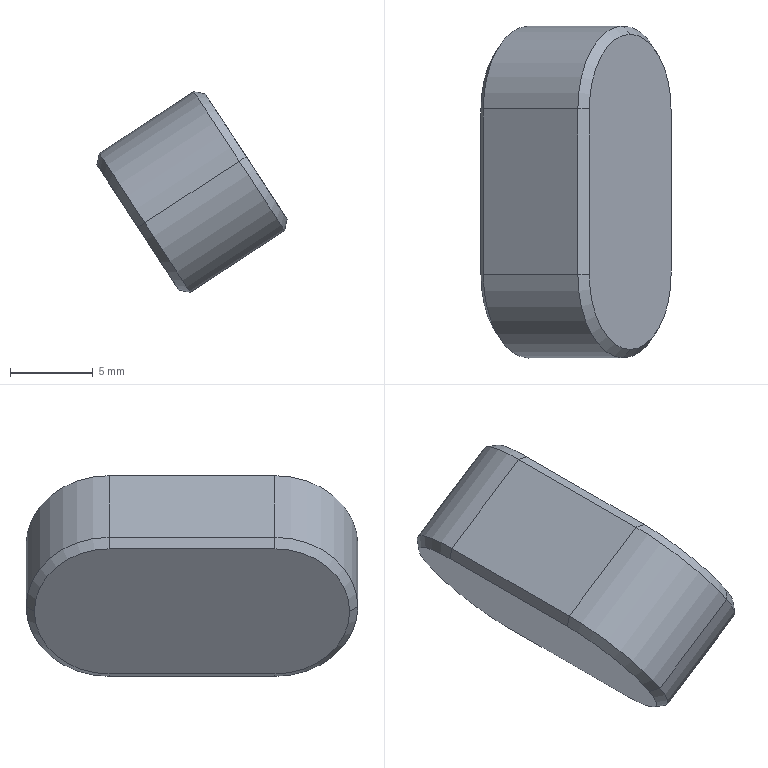Part | NX | features BREP 1 | 1 solid | 20 faces | box 11.452 x 20 x 12.091 mm | volume 1380 mm3 | plane 8 | cone 8 | cylinder 4 | commonest cylinder face diameters 10 x4
STEP:
#1=CARTESIAN_POINT('',(143.048,321.,299.856));
#2=VERTEX_POINT('',#1);
#3=CARTESIAN_POINT('',(140.587,325.5,303.624));
#4=VERTEX_POINT('',#3);
#5=CARTESIAN_POINT('',(140.587,321.,303.624));
#6=DIRECTION('',(0.8372,0.,0.5469));
#7=DIRECTION('',(0.5469,0.,-0.8372));
#8=AXIS2_PLACEMENT_3D('',#5,#6,#7);
#9=CIRCLE('',#8,4.5);
#10=EDGE_CURVE('',#2,#4,#9,.T.);
#11=ORIENTED_EDGE('',*,*,#10,.F.);
#12=CARTESIAN_POINT('',(143.048,311.,299.856));
#13=VERTEX_POINT('',#12);
#14=CARTESIAN_POINT('',(143.048,316.,299.856));
#15=DIRECTION('',(0.,1.,0.));
#16=VECTOR('',#15,1000.);
#17=LINE('',#14,#16);
#18=EDGE_CURVE('',#13,#2,#17,.T.);
#19=ORIENTED_EDGE('',*,*,#18,.F.);
#20=CARTESIAN_POINT('',(140.587,306.5,303.624));
#21=VERTEX_POINT('',#20);
#22=CARTESIAN_POINT('',(140.587,311.,303.624));
#23=DIRECTION('',(0.8372,0.,0.5469));
#24=DIRECTION('',(0.5469,0.,-0.8372));
#25=AXIS2_PLACEMENT_3D('',#22,#23,#24);
#26=CIRCLE('',#25,4.5);
#27=EDGE_CURVE('',#21,#13,#26,.T.);
#28=ORIENTED_EDGE('',*,*,#27,.F.);
#29=CARTESIAN_POINT('',(138.126,311.,307.391));
#30=VERTEX_POINT('',#29);
#31=CARTESIAN_POINT('',(140.587,311.,303.624));
#32=DIRECTION('',(0.8372,0.,0.5469));
#33=DIRECTION('',(0.5469,0.,-0.8372));
#34=AXIS2_PLACEMENT_3D('',#31,#32,#33);
#35=CIRCLE('',#34,4.5);
#36=EDGE_CURVE('',#30,#21,#35,.T.);
#37=ORIENTED_EDGE('',*,*,#36,.F.);
#38=CARTESIAN_POINT('',(138.126,321.,307.391));
#39=VERTEX_POINT('',#38);
#40=CARTESIAN_POINT('',(138.126,316.,307.391));
#41=DIRECTION('',(0.,-1.,0.));
#42=VECTOR('',#41,1000.);
#43=LINE('',#40,#42);
#44=EDGE_CURVE('',#39,#30,#43,.T.);
#45=ORIENTED_EDGE('',*,*,#44,.F.);
#46=CARTESIAN_POINT('',(140.587,321.,303.624));
#47=DIRECTION('',(0.8372,0.,0.5469));
#48=DIRECTION('',(0.5469,0.,-0.8372));
#49=AXIS2_PLACEMENT_3D('',#46,#47,#48);
#50=CIRCLE('',#49,4.5);
#51=EDGE_CURVE('',#4,#39,#50,.T.);
#52=ORIENTED_EDGE('',*,*,#51,.F.);
#53=EDGE_LOOP('',(#11,#19,#28,#37,#45,#52));
#54=FACE_BOUND('',#53,.T.);
#55=CARTESIAN_POINT('',(237.555,0.,155.201));
#56=DIRECTION('',(0.8372,0.,0.5469));
#57=DIRECTION('',(0.,-1.,0.));
#58=AXIS2_PLACEMENT_3D('',#55,#56,#57);
#59=PLANE('',#58);
#60=ADVANCED_FACE('',(#54),#59,.F.);
#61=CARTESIAN_POINT('',(141.005,326.,303.897));
#62=VERTEX_POINT('',#61);
#63=CARTESIAN_POINT('',(140.796,325.75,303.76));
#64=DIRECTION('',(-0.592,-0.7071,-0.3867));
#65=VECTOR('',#64,1000.);
#66=LINE('',#63,#65);
#67=EDGE_CURVE('',#62,#4,#66,.T.);
#68=ORIENTED_EDGE('',*,*,#67,.T.);
#69=ORIENTED_EDGE('',*,*,#51,.T.);
#70=CARTESIAN_POINT('',(138.271,321.,308.083));
#71=VERTEX_POINT('',#70);
#72=CARTESIAN_POINT('',(138.198,321.,307.737));
#73=DIRECTION('',(-0.2052,-0.000000081,-0.9787));
#74=VECTOR('',#73,1000.);
#75=LINE('',#72,#74);
#76=EDGE_CURVE('',#71,#39,#75,.T.);
#77=ORIENTED_EDGE('',*,*,#76,.F.);
#78=CARTESIAN_POINT('',(141.005,321.,303.897));
#79=DIRECTION('',(0.8372,0.,0.5469));
#80=DIRECTION('',(0.5469,0.,-0.8372));
#81=AXIS2_PLACEMENT_3D('',#78,#79,#80);
#82=CIRCLE('',#81,5.);
#83=EDGE_CURVE('',#62,#71,#82,.T.);
#84=ORIENTED_EDGE('',*,*,#83,.F.);
#85=EDGE_LOOP('',(#68,#69,#77,#84));
#86=FACE_BOUND('',#85,.T.);
#87=CARTESIAN_POINT('',(136.82,321.,301.162));
#88=DIRECTION('',(0.8372,0.,0.5469));
#89=DIRECTION('',(-0.2779,-0.8613,0.4254));
#90=AXIS2_PLACEMENT_3D('',#87,#88,#89);
#91=CONICAL_SURFACE('',#90,0.,0.7854);
#92=ADVANCED_FACE('',(#86),#91,.T.);
#93=ORIENTED_EDGE('',*,*,#76,.T.);
#94=ORIENTED_EDGE('',*,*,#44,.T.);
#95=CARTESIAN_POINT('',(138.271,311.,308.083));
#96=VERTEX_POINT('',#95);
#97=CARTESIAN_POINT('',(138.198,311.,307.737));
#98=DIRECTION('',(-0.2052,0.,-0.9787));
#99=VECTOR('',#98,1000.);
#100=LINE('',#97,#99);
#101=EDGE_CURVE('',#96,#30,#100,.T.);
#102=ORIENTED_EDGE('',*,*,#101,.F.);
#103=CARTESIAN_POINT('',(138.271,316.,308.083));
#104=DIRECTION('',(0.,-1.,0.));
#105=VECTOR('',#104,1000.);
#106=LINE('',#103,#105);
#107=EDGE_CURVE('',#71,#96,#106,.T.);
#108=ORIENTED_EDGE('',*,*,#107,.F.);
#109=EDGE_LOOP('',(#93,#94,#102,#108));
#110=FACE_BOUND('',#109,.T.);
#111=CARTESIAN_POINT('',(138.126,330.,307.391));
#112=DIRECTION('',(-0.9787,0.,0.2052));
#113=DIRECTION('',(0.,1.,0.));
#114=AXIS2_PLACEMENT_3D('',#111,#112,#113);
#115=PLANE('',#114);
#116=ADVANCED_FACE('',(#110),#115,.T.);
#117=ORIENTED_EDGE('',*,*,#101,.T.);
#118=ORIENTED_EDGE('',*,*,#36,.T.);
#119=CARTESIAN_POINT('',(141.005,306.,303.897));
#120=VERTEX_POINT('',#119);
#121=CARTESIAN_POINT('',(140.796,306.25,303.76));
#122=DIRECTION('',(-0.592,0.7071,-0.3867));
#123=VECTOR('',#122,1000.);
#124=LINE('',#121,#123);
#125=EDGE_CURVE('',#120,#21,#124,.T.);
#126=ORIENTED_EDGE('',*,*,#125,.F.);
#127=CARTESIAN_POINT('',(141.005,311.,303.897));
#128=DIRECTION('',(0.8372,0.,0.5469));
#129=DIRECTION('',(0.5469,0.,-0.8372));
#130=AXIS2_PLACEMENT_3D('',#127,#128,#129);
#131=CIRCLE('',#130,5.);
#132=EDGE_CURVE('',#96,#120,#131,.T.);
#133=ORIENTED_EDGE('',*,*,#132,.F.);
#134=EDGE_LOOP('',(#117,#118,#126,#133));
#135=FACE_BOUND('',#134,.T.);
#136=CARTESIAN_POINT('',(136.82,311.,301.162));
#137=DIRECTION('',(0.8372,0.,0.5469));
#138=DIRECTION('',(0.471,-0.5084,-0.7209));
#139=AXIS2_PLACEMENT_3D('',#136,#137,#138);
#140=CONICAL_SURFACE('',#139,0.,0.7854);
#141=ADVANCED_FACE('',(#135),#140,.T.);
#142=ORIENTED_EDGE('',*,*,#125,.T.);
#143=ORIENTED_EDGE('',*,*,#27,.T.);
#144=CARTESIAN_POINT('',(143.74,311.,299.711));
#145=VERTEX_POINT('',#144);
#146=CARTESIAN_POINT('',(143.394,311.,299.784));
#147=DIRECTION('',(-0.9787,0.000000064,0.2052));
#148=VECTOR('',#147,1000.);
#149=LINE('',#146,#148);
#150=EDGE_CURVE('',#145,#13,#149,.T.);
#151=ORIENTED_EDGE('',*,*,#150,.F.);
#152=CARTESIAN_POINT('',(141.005,311.,303.897));
#153=DIRECTION('',(0.8372,0.,0.5469));
#154=DIRECTION('',(0.5469,0.,-0.8372));
#155=AXIS2_PLACEMENT_3D('',#152,#153,#154);
#156=CIRCLE('',#155,5.);
#157=EDGE_CURVE('',#120,#145,#156,.T.);
#158=ORIENTED_EDGE('',*,*,#157,.F.);
#159=EDGE_LOOP('',(#142,#143,#151,#158));
#160=FACE_BOUND('',#159,.T.);
#161=CARTESIAN_POINT('',(136.82,311.,301.162));
#162=DIRECTION('',(0.8372,0.,0.5469));
#163=DIRECTION('',(0.2779,0.8613,-0.4254));
#164=AXIS2_PLACEMENT_3D('',#161,#162,#163);
#165=CONICAL_SURFACE('',#164,0.,0.7854);
#166=ADVANCED_FACE('',(#160),#165,.T.);
#167=ORIENTED_EDGE('',*,*,#150,.T.);
#168=ORIENTED_EDGE('',*,*,#18,.T.);
#169=CARTESIAN_POINT('',(143.74,321.,299.711));
#170=VERTEX_POINT('',#169);
#171=CARTESIAN_POINT('',(143.394,321.,299.784));
#172=DIRECTION('',(-0.9787,0.,0.2052));
#173=VECTOR('',#172,1000.);
#174=LINE('',#171,#173);
#175=EDGE_CURVE('',#170,#2,#174,.T.);
#176=ORIENTED_EDGE('',*,*,#175,.F.);
#177=CARTESIAN_POINT('',(143.74,316.,299.711));
#178=DIRECTION('',(0.,1.,0.));
#179=VECTOR('',#178,1000.);
#180=LINE('',#177,#179);
#181=EDGE_CURVE('',#145,#170,#180,.T.);
#182=ORIENTED_EDGE('',*,*,#181,.F.);
#183=EDGE_LOOP('',(#167,#168,#176,#182));
#184=FACE_BOUND('',#183,.T.);
#185=CARTESIAN_POINT('',(143.048,302.,299.856));
#186=DIRECTION('',(-0.2052,0.,-0.9787));
#187=DIRECTION('',(0.,-1.,0.));
#188=AXIS2_PLACEMENT_3D('',#185,#186,#187);
#189=PLANE('',#188);
#190=ADVANCED_FACE('',(#184),#189,.T.);
#191=ORIENTED_EDGE('',*,*,#175,.T.);
#192=ORIENTED_EDGE('',*,*,#10,.T.);
#193=ORIENTED_EDGE('',*,*,#67,.F.);
#194=CARTESIAN_POINT('',(141.005,321.,303.897));
#195=DIRECTION('',(0.8372,0.,0.5469));
#196=DIRECTION('',(0.5469,0.,-0.8372));
#197=AXIS2_PLACEMENT_3D('',#194,#195,#196);
#198=CIRCLE('',#197,5.);
#199=EDGE_CURVE('',#170,#62,#198,.T.);
#200=ORIENTED_EDGE('',*,*,#199,.F.);
#201=EDGE_LOOP('',(#191,#192,#193,#200));
#202=FACE_BOUND('',#201,.T.);
#203=CARTESIAN_POINT('',(136.82,321.,301.162));
#204=DIRECTION('',(0.8372,0.,0.5469));
#205=DIRECTION('',(-0.471,0.5084,0.7209));
#206=AXIS2_PLACEMENT_3D('',#203,#204,#205);
#207=CONICAL_SURFACE('',#206,0.,0.7854);
#208=ADVANCED_FACE('',(#202),#207,.T.);
#209=CARTESIAN_POINT('',(144.656,311.,311.657));
#210=VERTEX_POINT('',#209);
#211=CARTESIAN_POINT('',(144.656,321.,311.657));
#212=VERTEX_POINT('',#211);
#213=CARTESIAN_POINT('',(144.656,316.,311.657));
#214=DIRECTION('',(0.,1.,0.));
#215=VECTOR('',#214,1000.);
#216=LINE('',#213,#215);
#217=EDGE_CURVE('',#210,#212,#216,.T.);
#218=ORIENTED_EDGE('',*,*,#217,.F.);
#219=CARTESIAN_POINT('',(147.117,306.5,307.89));
#220=VERTEX_POINT('',#219);
#221=CARTESIAN_POINT('',(147.117,311.,307.89));
#222=DIRECTION('',(-0.8372,0.,-0.5469));
#223=DIRECTION('',(0.5469,0.,-0.8372));
#224=AXIS2_PLACEMENT_3D('',#221,#222,#223);
#225=CIRCLE('',#224,4.5);
#226=EDGE_CURVE('',#220,#210,#225,.T.);
#227=ORIENTED_EDGE('',*,*,#226,.F.);
#228=CARTESIAN_POINT('',(149.578,311.,304.122));
#229=VERTEX_POINT('',#228);
#230=CARTESIAN_POINT('',(147.117,311.,307.89));
#231=DIRECTION('',(-0.8372,0.,-0.5469));
#232=DIRECTION('',(0.5469,0.,-0.8372));
#233=AXIS2_PLACEMENT_3D('',#230,#231,#232);
#234=CIRCLE('',#233,4.5);
#235=EDGE_CURVE('',#229,#220,#234,.T.);
#236=ORIENTED_EDGE('',*,*,#235,.F.);
#237=CARTESIAN_POINT('',(149.578,321.,304.122));
#238=VERTEX_POINT('',#237);
#239=CARTESIAN_POINT('',(149.578,316.,304.122));
#240=DIRECTION('',(0.,-1.,0.));
#241=VECTOR('',#240,1000.);
#242=LINE('',#239,#241);
#243=EDGE_CURVE('',#238,#229,#242,.T.);
#244=ORIENTED_EDGE('',*,*,#243,.F.);
#245=CARTESIAN_POINT('',(147.117,325.5,307.89));
#246=VERTEX_POINT('',#245);
#247=CARTESIAN_POINT('',(147.117,321.,307.89));
#248=DIRECTION('',(-0.8372,0.,-0.5469));
#249=DIRECTION('',(0.5469,0.,-0.8372));
#250=AXIS2_PLACEMENT_3D('',#247,#248,#249);
#251=CIRCLE('',#250,4.5);
#252=EDGE_CURVE('',#246,#238,#251,.T.);
#253=ORIENTED_EDGE('',*,*,#252,.F.);
#254=CARTESIAN_POINT('',(147.117,321.,307.89));
#255=DIRECTION('',(-0.8372,0.,-0.5469));
#256=DIRECTION('',(0.5469,0.,-0.8372));
#257=AXIS2_PLACEMENT_3D('',#254,#255,#256);
#258=CIRCLE('',#257,4.5);
#259=EDGE_CURVE('',#212,#246,#258,.T.);
#260=ORIENTED_EDGE('',*,*,#259,.F.);
#261=EDGE_LOOP('',(#218,#227,#236,#244,#253,#260));
#262=FACE_BOUND('',#261,.T.);
#263=CARTESIAN_POINT('',(244.085,0.,159.467));
#264=DIRECTION('',(0.8372,0.,0.5469));
#265=DIRECTION('',(0.,-1.,0.));
#266=AXIS2_PLACEMENT_3D('',#263,#264,#265);
#267=PLANE('',#266);
#268=ADVANCED_FACE('',(#262),#267,.T.);
#269=CARTESIAN_POINT('',(146.698,306.,307.616));
#270=VERTEX_POINT('',#269);
#271=CARTESIAN_POINT('',(143.852,306.,305.757));
#272=DIRECTION('',(-0.8372,0.,-0.5469));
#273=VECTOR('',#272,1000.);
#274=LINE('',#271,#273);
#275=EDGE_CURVE('',#270,#120,#274,.T.);
#276=ORIENTED_EDGE('',*,*,#275,.T.);
#277=ORIENTED_EDGE('',*,*,#157,.T.);
#278=CARTESIAN_POINT('',(149.433,311.,303.43));
#279=VERTEX_POINT('',#278);
#280=CARTESIAN_POINT('',(146.587,311.,301.571));
#281=DIRECTION('',(-0.8372,0.,-0.5469));
#282=VECTOR('',#281,1000.);
#283=LINE('',#280,#282);
#284=EDGE_CURVE('',#279,#145,#283,.T.);
#285=ORIENTED_EDGE('',*,*,#284,.F.);
#286=CARTESIAN_POINT('',(146.698,311.,307.616));
#287=DIRECTION('',(-0.8372,0.,-0.5469));
#288=DIRECTION('',(0.5469,0.,-0.8372));
#289=AXIS2_PLACEMENT_3D('',#286,#287,#288);
#290=CIRCLE('',#289,5.);
#291=EDGE_CURVE('',#279,#270,#290,.T.);
#292=ORIENTED_EDGE('',*,*,#291,.T.);
#293=EDGE_LOOP('',(#276,#277,#285,#292));
#294=FACE_BOUND('',#293,.T.);
#295=CARTESIAN_POINT('',(143.852,311.,305.757));
#296=DIRECTION('',(-0.8372,0.,-0.5469));
#297=DIRECTION('',(-0.5469,0.,0.8372));
#298=AXIS2_PLACEMENT_3D('',#295,#296,#297);
#299=CYLINDRICAL_SURFACE('',#298,5.);
#300=ADVANCED_FACE('',(#294),#299,.T.);
#301=CARTESIAN_POINT('',(143.963,311.,311.802));
#302=VERTEX_POINT('',#301);
#303=CARTESIAN_POINT('',(141.117,311.,309.942));
#304=DIRECTION('',(-0.8372,0.,-0.5469));
#305=VECTOR('',#304,1000.);
#306=LINE('',#303,#305);
#307=EDGE_CURVE('',#302,#96,#306,.T.);
#308=ORIENTED_EDGE('',*,*,#307,.T.);
#309=ORIENTED_EDGE('',*,*,#132,.T.);
#310=ORIENTED_EDGE('',*,*,#275,.F.);
#311=CARTESIAN_POINT('',(146.698,311.,307.616));
#312=DIRECTION('',(-0.8372,0.,-0.5469));
#313=DIRECTION('',(0.5469,0.,-0.8372));
#314=AXIS2_PLACEMENT_3D('',#311,#312,#313);
#315=CIRCLE('',#314,5.);
#316=EDGE_CURVE('',#270,#302,#315,.T.);
#317=ORIENTED_EDGE('',*,*,#316,.T.);
#318=EDGE_LOOP('',(#308,#309,#310,#317));
#319=FACE_BOUND('',#318,.T.);
#320=CARTESIAN_POINT('',(143.852,311.,305.757));
#321=DIRECTION('',(-0.8372,0.,-0.5469));
#322=DIRECTION('',(0.,1.,0.));
#323=AXIS2_PLACEMENT_3D('',#320,#321,#322);
#324=CYLINDRICAL_SURFACE('',#323,5.);
#325=ADVANCED_FACE('',(#319),#324,.T.);
#326=CARTESIAN_POINT('',(143.963,321.,311.802));
#327=VERTEX_POINT('',#326);
#328=CARTESIAN_POINT('',(141.117,321.,309.942));
#329=DIRECTION('',(-0.8372,0.,-0.5469));
#330=VECTOR('',#329,1000.);
#331=LINE('',#328,#330);
#332=EDGE_CURVE('',#327,#71,#331,.T.);
#333=ORIENTED_EDGE('',*,*,#332,.T.);
#334=ORIENTED_EDGE('',*,*,#107,.T.);
#335=ORIENTED_EDGE('',*,*,#307,.F.);
#336=CARTESIAN_POINT('',(143.963,316.,311.802));
#337=DIRECTION('',(0.,1.,0.));
#338=VECTOR('',#337,1000.);
#339=LINE('',#336,#338);
#340=EDGE_CURVE('',#302,#327,#339,.T.);
#341=ORIENTED_EDGE('',*,*,#340,.T.);
#342=EDGE_LOOP('',(#333,#334,#335,#341));
#343=FACE_BOUND('',#342,.T.);
#344=CARTESIAN_POINT('',(144.382,306.,312.076));
#345=DIRECTION('',(-0.5469,0.,0.8372));
#346=DIRECTION('',(0.,-1.,0.));
#347=AXIS2_PLACEMENT_3D('',#344,#345,#346);
#348=PLANE('',#347);
#349=ADVANCED_FACE('',(#343),#348,.T.);
#350=CARTESIAN_POINT('',(146.698,326.,307.616));
#351=VERTEX_POINT('',#350);
#352=CARTESIAN_POINT('',(143.852,326.,305.757));
#353=DIRECTION('',(-0.8372,0.,-0.5469));
#354=VECTOR('',#353,1000.);
#355=LINE('',#352,#354);
#356=EDGE_CURVE('',#351,#62,#355,.T.);
#357=ORIENTED_EDGE('',*,*,#356,.T.);
#358=ORIENTED_EDGE('',*,*,#83,.T.);
#359=ORIENTED_EDGE('',*,*,#332,.F.);
#360=CARTESIAN_POINT('',(146.698,321.,307.616));
#361=DIRECTION('',(-0.8372,0.,-0.5469));
#362=DIRECTION('',(0.5469,0.,-0.8372));
#363=AXIS2_PLACEMENT_3D('',#360,#361,#362);
#364=CIRCLE('',#363,5.);
#365=EDGE_CURVE('',#327,#351,#364,.T.);
#366=ORIENTED_EDGE('',*,*,#365,.T.);
#367=EDGE_LOOP('',(#357,#358,#359,#366));
#368=FACE_BOUND('',#367,.T.);
#369=CARTESIAN_POINT('',(143.852,321.,305.757));
#370=DIRECTION('',(-0.8372,0.,-0.5469));
#371=DIRECTION('',(0.5469,0.,-0.8372));
#372=AXIS2_PLACEMENT_3D('',#369,#370,#371);
#373=CYLINDRICAL_SURFACE('',#372,5.);
#374=ADVANCED_FACE('',(#368),#373,.T.);
#375=ORIENTED_EDGE('',*,*,#284,.T.);
#376=ORIENTED_EDGE('',*,*,#181,.T.);
#377=CARTESIAN_POINT('',(149.433,321.,303.43));
#378=VERTEX_POINT('',#377);
#379=CARTESIAN_POINT('',(146.587,321.,301.571));
#380=DIRECTION('',(-0.8372,0.,-0.5469));
#381=VECTOR('',#380,1000.);
#382=LINE('',#379,#381);
#383=EDGE_CURVE('',#378,#170,#382,.T.);
#384=ORIENTED_EDGE('',*,*,#383,.F.);
#385=CARTESIAN_POINT('',(149.433,316.,303.43));
#386=DIRECTION('',(0.,-1.,0.));
#387=VECTOR('',#386,1000.);
#388=LINE('',#385,#387);
#389=EDGE_CURVE('',#378,#279,#388,.T.);
#390=ORIENTED_EDGE('',*,*,#389,.T.);
#391=EDGE_LOOP('',(#375,#376,#384,#390));
#392=FACE_BOUND('',#391,.T.);
#393=CARTESIAN_POINT('',(149.852,326.,303.704));
#394=DIRECTION('',(0.5469,0.,-0.8372));
#395=DIRECTION('',(0.,1.,0.));
#396=AXIS2_PLACEMENT_3D('',#393,#394,#395);
#397=PLANE('',#396);
#398=ADVANCED_FACE('',(#392),#397,.T.);
#399=ORIENTED_EDGE('',*,*,#383,.T.);
#400=ORIENTED_EDGE('',*,*,#199,.T.);
#401=ORIENTED_EDGE('',*,*,#356,.F.);
#402=CARTESIAN_POINT('',(146.698,321.,307.616));
#403=DIRECTION('',(-0.8372,0.,-0.5469));
#404=DIRECTION('',(0.5469,0.,-0.8372));
#405=AXIS2_PLACEMENT_3D('',#402,#403,#404);
#406=CIRCLE('',#405,5.);
#407=EDGE_CURVE('',#351,#378,#406,.T.);
#408=ORIENTED_EDGE('',*,*,#407,.T.);
#409=EDGE_LOOP('',(#399,#400,#401,#408));
#410=FACE_BOUND('',#409,.T.);
#411=CARTESIAN_POINT('',(143.852,321.,305.757));
#412=DIRECTION('',(-0.8372,0.,-0.5469));
#413=DIRECTION('',(0.,-1.,0.));
#414=AXIS2_PLACEMENT_3D('',#411,#412,#413);
#415=CYLINDRICAL_SURFACE('',#414,5.);
#416=ADVANCED_FACE('',(#410),#415,.T.);
#417=CARTESIAN_POINT('',(144.31,321.,311.73));
#418=DIRECTION('',(0.9787,-0.000000081,-0.2052));
#419=VECTOR('',#418,1000.);
#420=LINE('',#417,#419);
#421=EDGE_CURVE('',#327,#212,#420,.T.);
#422=ORIENTED_EDGE('',*,*,#421,.T.);
#423=ORIENTED_EDGE('',*,*,#259,.T.);
#424=CARTESIAN_POINT('',(146.908,325.75,307.753));
#425=DIRECTION('',(0.592,-0.7071,0.3867));
#426=VECTOR('',#425,1000.);
#427=LINE('',#424,#426);
#428=EDGE_CURVE('',#351,#246,#427,.T.);
#429=ORIENTED_EDGE('',*,*,#428,.F.);
#430=ORIENTED_EDGE('',*,*,#365,.F.);
#431=EDGE_LOOP('',(#422,#423,#429,#430));
#432=FACE_BOUND('',#431,.T.);
#433=CARTESIAN_POINT('',(150.884,321.,310.351));
#434=DIRECTION('',(-0.8372,0.,-0.5469));
#435=DIRECTION('',(-0.2779,-0.8613,0.4254));
#436=AXIS2_PLACEMENT_3D('',#433,#434,#435);
#437=CONICAL_SURFACE('',#436,0.,0.7854);
#438=ADVANCED_FACE('',(#432),#437,.T.);
#439=ORIENTED_EDGE('',*,*,#428,.T.);
#440=ORIENTED_EDGE('',*,*,#252,.T.);
#441=CARTESIAN_POINT('',(149.505,321.,303.776));
#442=DIRECTION('',(0.2052,-0.000000075,0.9787));
#443=VECTOR('',#442,1000.);
#444=LINE('',#441,#443);
#445=EDGE_CURVE('',#378,#238,#444,.T.);
#446=ORIENTED_EDGE('',*,*,#445,.F.);
#447=ORIENTED_EDGE('',*,*,#407,.F.);
#448=EDGE_LOOP('',(#439,#440,#446,#447));
#449=FACE_BOUND('',#448,.T.);
#450=CARTESIAN_POINT('',(150.884,321.,310.351));
#451=DIRECTION('',(-0.8372,0.,-0.5469));
#452=DIRECTION('',(-0.471,0.5084,0.7209));
#453=AXIS2_PLACEMENT_3D('',#450,#451,#452);
#454=CONICAL_SURFACE('',#453,0.,0.7854);
#455=ADVANCED_FACE('',(#449),#454,.T.);
#456=ORIENTED_EDGE('',*,*,#445,.T.);
#457=ORIENTED_EDGE('',*,*,#243,.T.);
#458=CARTESIAN_POINT('',(149.505,311.,303.776));
#459=DIRECTION('',(0.2052,0.,0.9787));
#460=VECTOR('',#459,1000.);
#461=LINE('',#458,#460);
#462=EDGE_CURVE('',#279,#229,#461,.T.);
#463=ORIENTED_EDGE('',*,*,#462,.F.);
#464=ORIENTED_EDGE('',*,*,#389,.F.);
#465=EDGE_LOOP('',(#456,#457,#463,#464));
#466=FACE_BOUND('',#465,.T.);
#467=CARTESIAN_POINT('',(149.578,302.,304.122));
#468=DIRECTION('',(-0.9787,0.,0.2052));
#469=DIRECTION('',(0.,-1.,0.));
#470=AXIS2_PLACEMENT_3D('',#467,#468,#469);
#471=PLANE('',#470);
#472=ADVANCED_FACE('',(#466),#471,.F.);
#473=ORIENTED_EDGE('',*,*,#462,.T.);
#474=ORIENTED_EDGE('',*,*,#235,.T.);
#475=CARTESIAN_POINT('',(146.908,306.25,307.753));
#476=DIRECTION('',(0.592,0.7071,0.3867));
#477=VECTOR('',#476,1000.);
#478=LINE('',#475,#477);
#479=EDGE_CURVE('',#270,#220,#478,.T.);
#480=ORIENTED_EDGE('',*,*,#479,.F.);
#481=ORIENTED_EDGE('',*,*,#291,.F.);
#482=EDGE_LOOP('',(#473,#474,#480,#481));
#483=FACE_BOUND('',#482,.T.);
#484=CARTESIAN_POINT('',(150.884,311.,310.351));
#485=DIRECTION('',(-0.8372,0.,-0.5469));
#486=DIRECTION('',(0.2779,0.8613,-0.4254));
#487=AXIS2_PLACEMENT_3D('',#484,#485,#486);
#488=CONICAL_SURFACE('',#487,0.,0.7854);
#489=ADVANCED_FACE('',(#483),#488,.T.);
#490=ORIENTED_EDGE('',*,*,#479,.T.);
#491=ORIENTED_EDGE('',*,*,#226,.T.);
#492=CARTESIAN_POINT('',(144.31,311.,311.73));
#493=DIRECTION('',(0.9787,0.000000075,-0.2052));
#494=VECTOR('',#493,1000.);
#495=LINE('',#492,#494);
#496=EDGE_CURVE('',#302,#210,#495,.T.);
#497=ORIENTED_EDGE('',*,*,#496,.F.);
#498=ORIENTED_EDGE('',*,*,#316,.F.);
#499=EDGE_LOOP('',(#490,#491,#497,#498));
#500=FACE_BOUND('',#499,.T.);
#501=CARTESIAN_POINT('',(150.884,311.,310.351));
#502=DIRECTION('',(-0.8372,0.,-0.5469));
#503=DIRECTION('',(0.471,-0.5084,-0.7209));
#504=AXIS2_PLACEMENT_3D('',#501,#502,#503);
#505=CONICAL_SURFACE('',#504,0.,0.7854);
#506=ADVANCED_FACE('',(#500),#505,.T.);
#507=ORIENTED_EDGE('',*,*,#496,.T.);
#508=ORIENTED_EDGE('',*,*,#217,.T.);
#509=ORIENTED_EDGE('',*,*,#421,.F.);
#510=ORIENTED_EDGE('',*,*,#340,.F.);
#511=EDGE_LOOP('',(#507,#508,#509,#510));
#512=FACE_BOUND('',#511,.T.);
#513=CARTESIAN_POINT('',(144.656,330.,311.657));
#514=DIRECTION('',(-0.2052,0.,-0.9787));
#515=DIRECTION('',(0.,1.,0.));
#516=AXIS2_PLACEMENT_3D('',#513,#514,#515);
#517=PLANE('',#516);
#518=ADVANCED_FACE('',(#512),#517,.F.);
#519=CLOSED_SHELL('',(#60,#92,#116,#141,#166,#190,#208,#268,#300,#325,#349,#374,#398,#416,#438,#455,#472,#489,#506,#518));
#520=MANIFOLD_SOLID_BREP('',#519);
#521=(LENGTH_UNIT()NAMED_UNIT(*)SI_UNIT(.MILLI.,.METRE.));
#522=UNCERTAINTY_MEASURE_WITH_UNIT(LENGTH_MEASURE(0.00001),#521,'','');
#523=(NAMED_UNIT(*)PLANE_ANGLE_UNIT()SI_UNIT($,.RADIAN.));
#524=(NAMED_UNIT(*)SI_UNIT($,.STERADIAN.)SOLID_ANGLE_UNIT());
#525=(GEOMETRIC_REPRESENTATION_CONTEXT(3)GLOBAL_UNCERTAINTY_ASSIGNED_CONTEXT((#522))GLOBAL_UNIT_ASSIGNED_CONTEXT((#521,#523,#524))REPRESENTATION_CONTEXT('',''));
#526=ADVANCED_BREP_SHAPE_REPRESENTATION('',(#520),#525);